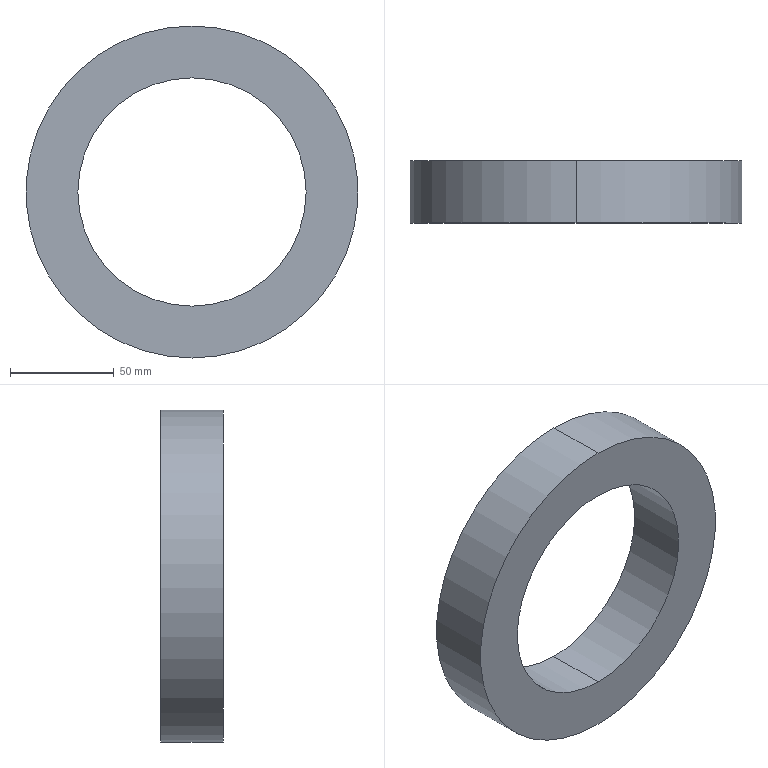Part | SolidWorks | features Extrusion 1, HoleWzd 1 | 1 solid | 30 faces | box 160 x 30 x 160 mm | volume 312871 mm3 | cone 16 | cylinder 12 | plane 2 | commonest cylinder face diameters 8.5 x8 110 x2 160 x2
STEP:
#1=CARTESIAN_POINT('',(65.,29.35,-4.25));
#2=VERTEX_POINT('',#1);
#3=CARTESIAN_POINT('',(65.,29.35,4.25));
#4=VERTEX_POINT('',#3);
#5=CARTESIAN_POINT('',(65.,29.35,0.));
#6=DIRECTION('',(0.,1.,0.));
#7=DIRECTION('',(0.,0.,1.));
#8=AXIS2_PLACEMENT_3D('',#5,#6,#7);
#9=CIRCLE('',#8,4.25);
#10=EDGE_CURVE('',#2,#4,#9,.T.);
#11=ORIENTED_EDGE('',*,*,#10,.F.);
#12=CARTESIAN_POINT('',(65.,30.,-5.025));
#13=VERTEX_POINT('',#12);
#14=CARTESIAN_POINT('',(65.,30.,-5.025));
#15=DIRECTION('',(0.,0.6428,-0.766));
#16=VECTOR('',#15,1000.);
#17=LINE('',#14,#16);
#18=EDGE_CURVE('',#2,#13,#17,.T.);
#19=ORIENTED_EDGE('',*,*,#18,.T.);
#20=CARTESIAN_POINT('',(65.,30.,5.025));
#21=VERTEX_POINT('',#20);
#22=CARTESIAN_POINT('',(65.,30.,0.));
#23=DIRECTION('',(0.,1.,0.));
#24=DIRECTION('',(0.,0.,1.));
#25=AXIS2_PLACEMENT_3D('',#22,#23,#24);
#26=CIRCLE('',#25,5.025);
#27=EDGE_CURVE('',#13,#21,#26,.T.);
#28=ORIENTED_EDGE('',*,*,#27,.T.);
#29=CARTESIAN_POINT('',(65.,30.,5.025));
#30=DIRECTION('',(0.,0.6428,0.766));
#31=VECTOR('',#30,1000.);
#32=LINE('',#29,#31);
#33=EDGE_CURVE('',#4,#21,#32,.T.);
#34=ORIENTED_EDGE('',*,*,#33,.F.);
#35=EDGE_LOOP('',(#11,#19,#28,#34));
#36=FACE_OUTER_BOUND('',#35,.T.);
#37=CARTESIAN_POINT('',(65.,30.,0.));
#38=DIRECTION('',(0.,1.,0.));
#39=DIRECTION('',(0.,0.,1.));
#40=AXIS2_PLACEMENT_3D('',#37,#38,#39);
#41=CONICAL_SURFACE('',#40,5.025,0.8727);
#42=ADVANCED_FACE('',(#36),#41,.F.);
#43=CARTESIAN_POINT('',(65.,8.,-4.25));
#44=VERTEX_POINT('',#43);
#45=CARTESIAN_POINT('',(65.,8.,4.25));
#46=VERTEX_POINT('',#45);
#47=CARTESIAN_POINT('',(65.,8.,0.));
#48=DIRECTION('',(0.,1.,0.));
#49=DIRECTION('',(0.,0.,1.));
#50=AXIS2_PLACEMENT_3D('',#47,#48,#49);
#51=CIRCLE('',#50,4.25);
#52=EDGE_CURVE('',#44,#46,#51,.T.);
#53=ORIENTED_EDGE('',*,*,#52,.F.);
#54=CARTESIAN_POINT('',(65.,30.,-4.25));
#55=DIRECTION('',(0.,1.,0.));
#56=VECTOR('',#55,1000.);
#57=LINE('',#54,#56);
#58=EDGE_CURVE('',#44,#2,#57,.T.);
#59=ORIENTED_EDGE('',*,*,#58,.T.);
#60=ORIENTED_EDGE('',*,*,#10,.T.);
#61=CARTESIAN_POINT('',(65.,30.,4.25));
#62=DIRECTION('',(0.,1.,0.));
#63=VECTOR('',#62,1000.);
#64=LINE('',#61,#63);
#65=EDGE_CURVE('',#46,#4,#64,.T.);
#66=ORIENTED_EDGE('',*,*,#65,.F.);
#67=EDGE_LOOP('',(#53,#59,#60,#66));
#68=FACE_OUTER_BOUND('',#67,.T.);
#69=CARTESIAN_POINT('',(65.,30.,0.));
#70=DIRECTION('',(0.,1.,0.));
#71=DIRECTION('',(0.,0.,1.));
#72=AXIS2_PLACEMENT_3D('',#69,#70,#71);
#73=CYLINDRICAL_SURFACE('',#72,4.25);
#74=ADVANCED_FACE('',(#68),#73,.F.);
#75=CARTESIAN_POINT('',(65.,5.446,0.));
#76=VERTEX_POINT('',#75);
#77=CARTESIAN_POINT('',(65.,8.,4.25));
#78=DIRECTION('',(0.,0.515,0.8572));
#79=VECTOR('',#78,1000.);
#80=LINE('',#77,#79);
#81=EDGE_CURVE('',#76,#46,#80,.T.);
#82=ORIENTED_EDGE('',*,*,#81,.F.);
#83=CARTESIAN_POINT('',(65.,8.,-4.25));
#84=DIRECTION('',(0.,0.515,-0.8572));
#85=VECTOR('',#84,1000.);
#86=LINE('',#83,#85);
#87=EDGE_CURVE('',#76,#44,#86,.T.);
#88=ORIENTED_EDGE('',*,*,#87,.T.);
#89=ORIENTED_EDGE('',*,*,#52,.T.);
#90=EDGE_LOOP('',(#82,#88,#89));
#91=FACE_OUTER_BOUND('',#90,.T.);
#92=CARTESIAN_POINT('',(65.,8.,0.));
#93=DIRECTION('',(0.,1.,0.));
#94=DIRECTION('',(0.,0.,1.));
#95=AXIS2_PLACEMENT_3D('',#92,#93,#94);
#96=CONICAL_SURFACE('',#95,4.25,1.03);
#97=ADVANCED_FACE('',(#91),#96,.F.);
#98=CARTESIAN_POINT('',(0.,29.35,60.75));
#99=VERTEX_POINT('',#98);
#100=CARTESIAN_POINT('',(0.,29.35,69.25));
#101=VERTEX_POINT('',#100);
#102=CARTESIAN_POINT('',(0.,29.35,65.));
#103=DIRECTION('',(0.,1.,0.));
#104=DIRECTION('',(0.,0.,1.));
#105=AXIS2_PLACEMENT_3D('',#102,#103,#104);
#106=CIRCLE('',#105,4.25);
#107=EDGE_CURVE('',#99,#101,#106,.T.);
#108=ORIENTED_EDGE('',*,*,#107,.F.);
#109=CARTESIAN_POINT('',(0.,30.,59.975));
#110=VERTEX_POINT('',#109);
#111=CARTESIAN_POINT('',(0.,30.,59.975));
#112=DIRECTION('',(0.,0.6428,-0.766));
#113=VECTOR('',#112,1000.);
#114=LINE('',#111,#113);
#115=EDGE_CURVE('',#99,#110,#114,.T.);
#116=ORIENTED_EDGE('',*,*,#115,.T.);
#117=CARTESIAN_POINT('',(0.,30.,70.025));
#118=VERTEX_POINT('',#117);
#119=CARTESIAN_POINT('',(0.,30.,65.));
#120=DIRECTION('',(0.,1.,0.));
#121=DIRECTION('',(0.,0.,1.));
#122=AXIS2_PLACEMENT_3D('',#119,#120,#121);
#123=CIRCLE('',#122,5.025);
#124=EDGE_CURVE('',#110,#118,#123,.T.);
#125=ORIENTED_EDGE('',*,*,#124,.T.);
#126=CARTESIAN_POINT('',(0.,30.,70.025));
#127=DIRECTION('',(0.,0.6428,0.766));
#128=VECTOR('',#127,1000.);
#129=LINE('',#126,#128);
#130=EDGE_CURVE('',#101,#118,#129,.T.);
#131=ORIENTED_EDGE('',*,*,#130,.F.);
#132=EDGE_LOOP('',(#108,#116,#125,#131));
#133=FACE_OUTER_BOUND('',#132,.T.);
#134=CARTESIAN_POINT('',(0.,30.,65.));
#135=DIRECTION('',(0.,1.,0.));
#136=DIRECTION('',(0.,0.,1.));
#137=AXIS2_PLACEMENT_3D('',#134,#135,#136);
#138=CONICAL_SURFACE('',#137,5.025,0.8727);
#139=ADVANCED_FACE('',(#133),#138,.F.);
#140=CARTESIAN_POINT('',(0.,8.,60.75));
#141=VERTEX_POINT('',#140);
#142=CARTESIAN_POINT('',(0.,8.,69.25));
#143=VERTEX_POINT('',#142);
#144=CARTESIAN_POINT('',(0.,8.,65.));
#145=DIRECTION('',(0.,1.,0.));
#146=DIRECTION('',(0.,0.,1.));
#147=AXIS2_PLACEMENT_3D('',#144,#145,#146);
#148=CIRCLE('',#147,4.25);
#149=EDGE_CURVE('',#141,#143,#148,.T.);
#150=ORIENTED_EDGE('',*,*,#149,.F.);
#151=CARTESIAN_POINT('',(0.,30.,60.75));
#152=DIRECTION('',(0.,1.,0.));
#153=VECTOR('',#152,1000.);
#154=LINE('',#151,#153);
#155=EDGE_CURVE('',#141,#99,#154,.T.);
#156=ORIENTED_EDGE('',*,*,#155,.T.);
#157=ORIENTED_EDGE('',*,*,#107,.T.);
#158=CARTESIAN_POINT('',(0.,30.,69.25));
#159=DIRECTION('',(0.,1.,0.));
#160=VECTOR('',#159,1000.);
#161=LINE('',#158,#160);
#162=EDGE_CURVE('',#143,#101,#161,.T.);
#163=ORIENTED_EDGE('',*,*,#162,.F.);
#164=EDGE_LOOP('',(#150,#156,#157,#163));
#165=FACE_OUTER_BOUND('',#164,.T.);
#166=CARTESIAN_POINT('',(0.,30.,65.));
#167=DIRECTION('',(0.,1.,0.));
#168=DIRECTION('',(0.,0.,1.));
#169=AXIS2_PLACEMENT_3D('',#166,#167,#168);
#170=CYLINDRICAL_SURFACE('',#169,4.25);
#171=ADVANCED_FACE('',(#165),#170,.F.);
#172=CARTESIAN_POINT('',(0.,5.446,65.));
#173=VERTEX_POINT('',#172);
#174=CARTESIAN_POINT('',(0.,8.,69.25));
#175=DIRECTION('',(0.,0.515,0.8572));
#176=VECTOR('',#175,1000.);
#177=LINE('',#174,#176);
#178=EDGE_CURVE('',#173,#143,#177,.T.);
#179=ORIENTED_EDGE('',*,*,#178,.F.);
#180=CARTESIAN_POINT('',(0.,8.,60.75));
#181=DIRECTION('',(0.,0.515,-0.8572));
#182=VECTOR('',#181,1000.);
#183=LINE('',#180,#182);
#184=EDGE_CURVE('',#173,#141,#183,.T.);
#185=ORIENTED_EDGE('',*,*,#184,.T.);
#186=ORIENTED_EDGE('',*,*,#149,.T.);
#187=EDGE_LOOP('',(#179,#185,#186));
#188=FACE_OUTER_BOUND('',#187,.T.);
#189=CARTESIAN_POINT('',(0.,8.,65.));
#190=DIRECTION('',(0.,1.,0.));
#191=DIRECTION('',(0.,0.,1.));
#192=AXIS2_PLACEMENT_3D('',#189,#190,#191);
#193=CONICAL_SURFACE('',#192,4.25,1.03);
#194=ADVANCED_FACE('',(#188),#193,.F.);
#195=CARTESIAN_POINT('',(-65.,29.35,-4.25));
#196=VERTEX_POINT('',#195);
#197=CARTESIAN_POINT('',(-65.,29.35,4.25));
#198=VERTEX_POINT('',#197);
#199=CARTESIAN_POINT('',(-65.,29.35,0.));
#200=DIRECTION('',(0.,1.,0.));
#201=DIRECTION('',(0.,0.,1.));
#202=AXIS2_PLACEMENT_3D('',#199,#200,#201);
#203=CIRCLE('',#202,4.25);
#204=EDGE_CURVE('',#196,#198,#203,.T.);
#205=ORIENTED_EDGE('',*,*,#204,.F.);
#206=CARTESIAN_POINT('',(-65.,30.,-5.025));
#207=VERTEX_POINT('',#206);
#208=CARTESIAN_POINT('',(-65.,30.,-5.025));
#209=DIRECTION('',(0.,0.6428,-0.766));
#210=VECTOR('',#209,1000.);
#211=LINE('',#208,#210);
#212=EDGE_CURVE('',#196,#207,#211,.T.);
#213=ORIENTED_EDGE('',*,*,#212,.T.);
#214=CARTESIAN_POINT('',(-65.,30.,5.025));
#215=VERTEX_POINT('',#214);
#216=CARTESIAN_POINT('',(-65.,30.,0.));
#217=DIRECTION('',(0.,1.,0.));
#218=DIRECTION('',(0.,0.,1.));
#219=AXIS2_PLACEMENT_3D('',#216,#217,#218);
#220=CIRCLE('',#219,5.025);
#221=EDGE_CURVE('',#207,#215,#220,.T.);
#222=ORIENTED_EDGE('',*,*,#221,.T.);
#223=CARTESIAN_POINT('',(-65.,30.,5.025));
#224=DIRECTION('',(0.,0.6428,0.766));
#225=VECTOR('',#224,1000.);
#226=LINE('',#223,#225);
#227=EDGE_CURVE('',#198,#215,#226,.T.);
#228=ORIENTED_EDGE('',*,*,#227,.F.);
#229=EDGE_LOOP('',(#205,#213,#222,#228));
#230=FACE_OUTER_BOUND('',#229,.T.);
#231=CARTESIAN_POINT('',(-65.,30.,0.));
#232=DIRECTION('',(0.,1.,0.));
#233=DIRECTION('',(0.,0.,1.));
#234=AXIS2_PLACEMENT_3D('',#231,#232,#233);
#235=CONICAL_SURFACE('',#234,5.025,0.8727);
#236=ADVANCED_FACE('',(#230),#235,.F.);
#237=CARTESIAN_POINT('',(-65.,8.,-4.25));
#238=VERTEX_POINT('',#237);
#239=CARTESIAN_POINT('',(-65.,8.,4.25));
#240=VERTEX_POINT('',#239);
#241=CARTESIAN_POINT('',(-65.,8.,0.));
#242=DIRECTION('',(0.,1.,0.));
#243=DIRECTION('',(0.,0.,1.));
#244=AXIS2_PLACEMENT_3D('',#241,#242,#243);
#245=CIRCLE('',#244,4.25);
#246=EDGE_CURVE('',#238,#240,#245,.T.);
#247=ORIENTED_EDGE('',*,*,#246,.F.);
#248=CARTESIAN_POINT('',(-65.,30.,-4.25));
#249=DIRECTION('',(0.,1.,0.));
#250=VECTOR('',#249,1000.);
#251=LINE('',#248,#250);
#252=EDGE_CURVE('',#238,#196,#251,.T.);
#253=ORIENTED_EDGE('',*,*,#252,.T.);
#254=ORIENTED_EDGE('',*,*,#204,.T.);
#255=CARTESIAN_POINT('',(-65.,30.,4.25));
#256=DIRECTION('',(0.,1.,0.));
#257=VECTOR('',#256,1000.);
#258=LINE('',#255,#257);
#259=EDGE_CURVE('',#240,#198,#258,.T.);
#260=ORIENTED_EDGE('',*,*,#259,.F.);
#261=EDGE_LOOP('',(#247,#253,#254,#260));
#262=FACE_OUTER_BOUND('',#261,.T.);
#263=CARTESIAN_POINT('',(-65.,30.,0.));
#264=DIRECTION('',(0.,1.,0.));
#265=DIRECTION('',(0.,0.,1.));
#266=AXIS2_PLACEMENT_3D('',#263,#264,#265);
#267=CYLINDRICAL_SURFACE('',#266,4.25);
#268=ADVANCED_FACE('',(#262),#267,.F.);
#269=CARTESIAN_POINT('',(-65.,5.446,0.));
#270=VERTEX_POINT('',#269);
#271=CARTESIAN_POINT('',(-65.,8.,4.25));
#272=DIRECTION('',(0.,0.515,0.8572));
#273=VECTOR('',#272,1000.);
#274=LINE('',#271,#273);
#275=EDGE_CURVE('',#270,#240,#274,.T.);
#276=ORIENTED_EDGE('',*,*,#275,.F.);
#277=CARTESIAN_POINT('',(-65.,8.,-4.25));
#278=DIRECTION('',(0.,0.515,-0.8572));
#279=VECTOR('',#278,1000.);
#280=LINE('',#277,#279);
#281=EDGE_CURVE('',#270,#238,#280,.T.);
#282=ORIENTED_EDGE('',*,*,#281,.T.);
#283=ORIENTED_EDGE('',*,*,#246,.T.);
#284=EDGE_LOOP('',(#276,#282,#283));
#285=FACE_OUTER_BOUND('',#284,.T.);
#286=CARTESIAN_POINT('',(-65.,8.,0.));
#287=DIRECTION('',(0.,1.,0.));
#288=DIRECTION('',(0.,0.,1.));
#289=AXIS2_PLACEMENT_3D('',#286,#287,#288);
#290=CONICAL_SURFACE('',#289,4.25,1.03);
#291=ADVANCED_FACE('',(#285),#290,.F.);
#292=CARTESIAN_POINT('',(0.,29.35,-69.25));
#293=VERTEX_POINT('',#292);
#294=CARTESIAN_POINT('',(0.,29.35,-60.75));
#295=VERTEX_POINT('',#294);
#296=CARTESIAN_POINT('',(0.,29.35,-65.));
#297=DIRECTION('',(0.,1.,0.));
#298=DIRECTION('',(0.,0.,1.));
#299=AXIS2_PLACEMENT_3D('',#296,#297,#298);
#300=CIRCLE('',#299,4.25);
#301=EDGE_CURVE('',#293,#295,#300,.T.);
#302=ORIENTED_EDGE('',*,*,#301,.F.);
#303=CARTESIAN_POINT('',(0.,30.,-70.025));
#304=VERTEX_POINT('',#303);
#305=CARTESIAN_POINT('',(0.,30.,-70.025));
#306=DIRECTION('',(0.,0.6428,-0.766));
#307=VECTOR('',#306,1000.);
#308=LINE('',#305,#307);
#309=EDGE_CURVE('',#293,#304,#308,.T.);
#310=ORIENTED_EDGE('',*,*,#309,.T.);
#311=CARTESIAN_POINT('',(0.,30.,-59.975));
#312=VERTEX_POINT('',#311);
#313=CARTESIAN_POINT('',(0.,30.,-65.));
#314=DIRECTION('',(0.,1.,0.));
#315=DIRECTION('',(0.,0.,1.));
#316=AXIS2_PLACEMENT_3D('',#313,#314,#315);
#317=CIRCLE('',#316,5.025);
#318=EDGE_CURVE('',#304,#312,#317,.T.);
#319=ORIENTED_EDGE('',*,*,#318,.T.);
#320=CARTESIAN_POINT('',(0.,30.,-59.975));
#321=DIRECTION('',(0.,0.6428,0.766));
#322=VECTOR('',#321,1000.);
#323=LINE('',#320,#322);
#324=EDGE_CURVE('',#295,#312,#323,.T.);
#325=ORIENTED_EDGE('',*,*,#324,.F.);
#326=EDGE_LOOP('',(#302,#310,#319,#325));
#327=FACE_OUTER_BOUND('',#326,.T.);
#328=CARTESIAN_POINT('',(0.,30.,-65.));
#329=DIRECTION('',(0.,1.,0.));
#330=DIRECTION('',(0.,0.,1.));
#331=AXIS2_PLACEMENT_3D('',#328,#329,#330);
#332=CONICAL_SURFACE('',#331,5.025,0.8727);
#333=ADVANCED_FACE('',(#327),#332,.F.);
#334=CARTESIAN_POINT('',(0.,8.,-69.25));
#335=VERTEX_POINT('',#334);
#336=CARTESIAN_POINT('',(0.,8.,-60.75));
#337=VERTEX_POINT('',#336);
#338=CARTESIAN_POINT('',(0.,8.,-65.));
#339=DIRECTION('',(0.,1.,0.));
#340=DIRECTION('',(0.,0.,1.));
#341=AXIS2_PLACEMENT_3D('',#338,#339,#340);
#342=CIRCLE('',#341,4.25);
#343=EDGE_CURVE('',#335,#337,#342,.T.);
#344=ORIENTED_EDGE('',*,*,#343,.F.);
#345=CARTESIAN_POINT('',(0.,30.,-69.25));
#346=DIRECTION('',(0.,1.,0.));
#347=VECTOR('',#346,1000.);
#348=LINE('',#345,#347);
#349=EDGE_CURVE('',#335,#293,#348,.T.);
#350=ORIENTED_EDGE('',*,*,#349,.T.);
#351=ORIENTED_EDGE('',*,*,#301,.T.);
#352=CARTESIAN_POINT('',(0.,30.,-60.75));
#353=DIRECTION('',(0.,1.,0.));
#354=VECTOR('',#353,1000.);
#355=LINE('',#352,#354);
#356=EDGE_CURVE('',#337,#295,#355,.T.);
#357=ORIENTED_EDGE('',*,*,#356,.F.);
#358=EDGE_LOOP('',(#344,#350,#351,#357));
#359=FACE_OUTER_BOUND('',#358,.T.);
#360=CARTESIAN_POINT('',(0.,30.,-65.));
#361=DIRECTION('',(0.,1.,0.));
#362=DIRECTION('',(0.,0.,1.));
#363=AXIS2_PLACEMENT_3D('',#360,#361,#362);
#364=CYLINDRICAL_SURFACE('',#363,4.25);
#365=ADVANCED_FACE('',(#359),#364,.F.);
#366=CARTESIAN_POINT('',(0.,5.446,-65.));
#367=VERTEX_POINT('',#366);
#368=CARTESIAN_POINT('',(0.,8.,-60.75));
#369=DIRECTION('',(0.,0.515,0.8572));
#370=VECTOR('',#369,1000.);
#371=LINE('',#368,#370);
#372=EDGE_CURVE('',#367,#337,#371,.T.);
#373=ORIENTED_EDGE('',*,*,#372,.F.);
#374=CARTESIAN_POINT('',(0.,8.,-69.25));
#375=DIRECTION('',(0.,0.515,-0.8572));
#376=VECTOR('',#375,1000.);
#377=LINE('',#374,#376);
#378=EDGE_CURVE('',#367,#335,#377,.T.);
#379=ORIENTED_EDGE('',*,*,#378,.T.);
#380=ORIENTED_EDGE('',*,*,#343,.T.);
#381=EDGE_LOOP('',(#373,#379,#380));
#382=FACE_OUTER_BOUND('',#381,.T.);
#383=CARTESIAN_POINT('',(0.,8.,-65.));
#384=DIRECTION('',(0.,1.,0.));
#385=DIRECTION('',(0.,0.,1.));
#386=AXIS2_PLACEMENT_3D('',#383,#384,#385);
#387=CONICAL_SURFACE('',#386,4.25,1.03);
#388=ADVANCED_FACE('',(#382),#387,.F.);
#389=CARTESIAN_POINT('',(0.,30.,-55.));
#390=VERTEX_POINT('',#389);
#391=CARTESIAN_POINT('',(0.,30.,55.));
#392=VERTEX_POINT('',#391);
#393=CARTESIAN_POINT('',(0.,30.,0.));
#394=DIRECTION('',(0.,1.,0.));
#395=DIRECTION('',(0.,0.,1.));
#396=AXIS2_PLACEMENT_3D('',#393,#394,#395);
#397=CIRCLE('',#396,55.);
#398=EDGE_CURVE('',#390,#392,#397,.T.);
#399=ORIENTED_EDGE('',*,*,#398,.T.);
#400=CARTESIAN_POINT('',(0.,0.,55.));
#401=VERTEX_POINT('',#400);
#402=CARTESIAN_POINT('',(0.,30.,55.));
#403=DIRECTION('',(0.,-1.,0.));
#404=VECTOR('',#403,1000.);
#405=LINE('',#402,#404);
#406=EDGE_CURVE('',#392,#401,#405,.T.);
#407=ORIENTED_EDGE('',*,*,#406,.T.);
#408=CARTESIAN_POINT('',(0.,0.,-55.));
#409=VERTEX_POINT('',#408);
#410=CARTESIAN_POINT('',(0.,0.,0.));
#411=DIRECTION('',(0.,1.,0.));
#412=DIRECTION('',(0.,0.,1.));
#413=AXIS2_PLACEMENT_3D('',#410,#411,#412);
#414=CIRCLE('',#413,55.);
#415=EDGE_CURVE('',#409,#401,#414,.T.);
#416=ORIENTED_EDGE('',*,*,#415,.F.);
#417=CARTESIAN_POINT('',(0.,30.,-55.));
#418=DIRECTION('',(0.,-1.,0.));
#419=VECTOR('',#418,1000.);
#420=LINE('',#417,#419);
#421=EDGE_CURVE('',#390,#409,#420,.T.);
#422=ORIENTED_EDGE('',*,*,#421,.F.);
#423=EDGE_LOOP('',(#399,#407,#416,#422));
#424=FACE_OUTER_BOUND('',#423,.T.);
#425=CARTESIAN_POINT('',(0.,30.,0.));
#426=DIRECTION('',(0.,-1.,0.));
#427=DIRECTION('',(0.,0.,-1.));
#428=AXIS2_PLACEMENT_3D('',#425,#426,#427);
#429=CYLINDRICAL_SURFACE('',#428,55.);
#430=ADVANCED_FACE('',(#424),#429,.F.);
#431=CARTESIAN_POINT('',(0.,30.,80.));
#432=VERTEX_POINT('',#431);
#433=CARTESIAN_POINT('',(0.,30.,-80.));
#434=VERTEX_POINT('',#433);
#435=CARTESIAN_POINT('',(0.,30.,0.));
#436=DIRECTION('',(0.,1.,0.));
#437=DIRECTION('',(0.,0.,1.));
#438=AXIS2_PLACEMENT_3D('',#435,#436,#437);
#439=CIRCLE('',#438,80.);
#440=EDGE_CURVE('',#432,#434,#439,.T.);
#441=ORIENTED_EDGE('',*,*,#440,.F.);
#442=CARTESIAN_POINT('',(0.,0.,80.));
#443=VERTEX_POINT('',#442);
#444=CARTESIAN_POINT('',(0.,30.,80.));
#445=DIRECTION('',(0.,-1.,0.));
#446=VECTOR('',#445,1000.);
#447=LINE('',#444,#446);
#448=EDGE_CURVE('',#432,#443,#447,.T.);
#449=ORIENTED_EDGE('',*,*,#448,.T.);
#450=CARTESIAN_POINT('',(0.,0.,-80.));
#451=VERTEX_POINT('',#450);
#452=CARTESIAN_POINT('',(0.,0.,0.));
#453=DIRECTION('',(0.,1.,0.));
#454=DIRECTION('',(0.,0.,1.));
#455=AXIS2_PLACEMENT_3D('',#452,#453,#454);
#456=CIRCLE('',#455,80.);
#457=EDGE_CURVE('',#443,#451,#456,.T.);
#458=ORIENTED_EDGE('',*,*,#457,.T.);
#459=CARTESIAN_POINT('',(0.,30.,-80.));
#460=DIRECTION('',(0.,-1.,0.));
#461=VECTOR('',#460,1000.);
#462=LINE('',#459,#461);
#463=EDGE_CURVE('',#434,#451,#462,.T.);
#464=ORIENTED_EDGE('',*,*,#463,.F.);
#465=EDGE_LOOP('',(#441,#449,#458,#464));
#466=FACE_OUTER_BOUND('',#465,.T.);
#467=CARTESIAN_POINT('',(0.,30.,0.));
#468=DIRECTION('',(0.,-1.,0.));
#469=DIRECTION('',(0.,0.,-1.));
#470=AXIS2_PLACEMENT_3D('',#467,#468,#469);
#471=CYLINDRICAL_SURFACE('',#470,80.);
#472=ADVANCED_FACE('',(#466),#471,.T.);
#473=CARTESIAN_POINT('',(65.,30.,0.));
#474=DIRECTION('',(0.,1.,0.));
#475=DIRECTION('',(0.,0.,1.));
#476=AXIS2_PLACEMENT_3D('',#473,#474,#475);
#477=CIRCLE('',#476,5.025);
#478=EDGE_CURVE('',#21,#13,#477,.T.);
#479=ORIENTED_EDGE('',*,*,#478,.F.);
#480=ORIENTED_EDGE('',*,*,#27,.F.);
#481=EDGE_LOOP('',(#479,#480));
#482=FACE_BOUND('',#481,.T.);
#483=CARTESIAN_POINT('',(0.,30.,65.));
#484=DIRECTION('',(0.,1.,0.));
#485=DIRECTION('',(0.,0.,1.));
#486=AXIS2_PLACEMENT_3D('',#483,#484,#485);
#487=CIRCLE('',#486,5.025);
#488=EDGE_CURVE('',#118,#110,#487,.T.);
#489=ORIENTED_EDGE('',*,*,#488,.F.);
#490=ORIENTED_EDGE('',*,*,#124,.F.);
#491=EDGE_LOOP('',(#489,#490));
#492=FACE_BOUND('',#491,.T.);
#493=CARTESIAN_POINT('',(-65.,30.,0.));
#494=DIRECTION('',(0.,1.,0.));
#495=DIRECTION('',(0.,0.,1.));
#496=AXIS2_PLACEMENT_3D('',#493,#494,#495);
#497=CIRCLE('',#496,5.025);
#498=EDGE_CURVE('',#215,#207,#497,.T.);
#499=ORIENTED_EDGE('',*,*,#498,.F.);
#500=ORIENTED_EDGE('',*,*,#221,.F.);
#501=EDGE_LOOP('',(#499,#500));
#502=FACE_BOUND('',#501,.T.);
#503=CARTESIAN_POINT('',(0.,30.,-65.));
#504=DIRECTION('',(0.,1.,0.));
#505=DIRECTION('',(0.,0.,1.));
#506=AXIS2_PLACEMENT_3D('',#503,#504,#505);
#507=CIRCLE('',#506,5.025);
#508=EDGE_CURVE('',#312,#304,#507,.T.);
#509=ORIENTED_EDGE('',*,*,#508,.F.);
#510=ORIENTED_EDGE('',*,*,#318,.F.);
#511=EDGE_LOOP('',(#509,#510));
#512=FACE_BOUND('',#511,.T.);
#513=CARTESIAN_POINT('',(0.,30.,0.));
#514=DIRECTION('',(0.,1.,0.));
#515=DIRECTION('',(0.,0.,1.));
#516=AXIS2_PLACEMENT_3D('',#513,#514,#515);
#517=CIRCLE('',#516,80.);
#518=EDGE_CURVE('',#434,#432,#517,.T.);
#519=ORIENTED_EDGE('',*,*,#518,.T.);
#520=ORIENTED_EDGE('',*,*,#440,.T.);
#521=EDGE_LOOP('',(#519,#520));
#522=FACE_OUTER_BOUND('',#521,.T.);
#523=ORIENTED_EDGE('',*,*,#398,.F.);
#524=CARTESIAN_POINT('',(0.,30.,0.));
#525=DIRECTION('',(0.,1.,0.));
#526=DIRECTION('',(0.,0.,1.));
#527=AXIS2_PLACEMENT_3D('',#524,#525,#526);
#528=CIRCLE('',#527,55.);
#529=EDGE_CURVE('',#392,#390,#528,.T.);
#530=ORIENTED_EDGE('',*,*,#529,.F.);
#531=EDGE_LOOP('',(#523,#530));
#532=FACE_BOUND('',#531,.T.);
#533=CARTESIAN_POINT('',(0.,30.,0.));
#534=DIRECTION('',(0.,1.,0.));
#535=DIRECTION('',(0.,0.,1.));
#536=AXIS2_PLACEMENT_3D('',#533,#534,#535);
#537=PLANE('',#536);
#538=ADVANCED_FACE('',(#482,#492,#502,#512,#522,#532),#537,.T.);
#539=CARTESIAN_POINT('',(0.,0.,0.));
#540=DIRECTION('',(0.,1.,0.));
#541=DIRECTION('',(0.,0.,1.));
#542=AXIS2_PLACEMENT_3D('',#539,#540,#541);
#543=CIRCLE('',#542,80.);
#544=EDGE_CURVE('',#451,#443,#543,.T.);
#545=ORIENTED_EDGE('',*,*,#544,.F.);
#546=ORIENTED_EDGE('',*,*,#457,.F.);
#547=EDGE_LOOP('',(#545,#546));
#548=FACE_OUTER_BOUND('',#547,.T.);
#549=ORIENTED_EDGE('',*,*,#415,.T.);
#550=CARTESIAN_POINT('',(0.,0.,0.));
#551=DIRECTION('',(0.,1.,0.));
#552=DIRECTION('',(0.,0.,1.));
#553=AXIS2_PLACEMENT_3D('',#550,#551,#552);
#554=CIRCLE('',#553,55.);
#555=EDGE_CURVE('',#401,#409,#554,.T.);
#556=ORIENTED_EDGE('',*,*,#555,.T.);
#557=EDGE_LOOP('',(#549,#556));
#558=FACE_BOUND('',#557,.T.);
#559=CARTESIAN_POINT('',(0.,0.,0.));
#560=DIRECTION('',(0.,1.,0.));
#561=DIRECTION('',(0.,0.,1.));
#562=AXIS2_PLACEMENT_3D('',#559,#560,#561);
#563=PLANE('',#562);
#564=ADVANCED_FACE('',(#548,#558),#563,.F.);
#565=ORIENTED_EDGE('',*,*,#448,.F.);
#566=ORIENTED_EDGE('',*,*,#518,.F.);
#567=ORIENTED_EDGE('',*,*,#463,.T.);
#568=ORIENTED_EDGE('',*,*,#544,.T.);
#569=EDGE_LOOP('',(#565,#566,#567,#568));
#570=FACE_OUTER_BOUND('',#569,.T.);
#571=CARTESIAN_POINT('',(0.,30.,0.));
#572=DIRECTION('',(0.,-1.,0.));
#573=DIRECTION('',(0.,0.,-1.));
#574=AXIS2_PLACEMENT_3D('',#571,#572,#573);
#575=CYLINDRICAL_SURFACE('',#574,80.);
#576=ADVANCED_FACE('',(#570),#575,.T.);
#577=ORIENTED_EDGE('',*,*,#406,.F.);
#578=ORIENTED_EDGE('',*,*,#529,.T.);
#579=ORIENTED_EDGE('',*,*,#421,.T.);
#580=ORIENTED_EDGE('',*,*,#555,.F.);
#581=EDGE_LOOP('',(#577,#578,#579,#580));
#582=FACE_OUTER_BOUND('',#581,.T.);
#583=CARTESIAN_POINT('',(0.,30.,0.));
#584=DIRECTION('',(0.,-1.,0.));
#585=DIRECTION('',(0.,0.,-1.));
#586=AXIS2_PLACEMENT_3D('',#583,#584,#585);
#587=CYLINDRICAL_SURFACE('',#586,55.);
#588=ADVANCED_FACE('',(#582),#587,.F.);
#589=ORIENTED_EDGE('',*,*,#378,.F.);
#590=ORIENTED_EDGE('',*,*,#372,.T.);
#591=CARTESIAN_POINT('',(0.,8.,-65.));
#592=DIRECTION('',(0.,1.,0.));
#593=DIRECTION('',(0.,0.,1.));
#594=AXIS2_PLACEMENT_3D('',#591,#592,#593);
#595=CIRCLE('',#594,4.25);
#596=EDGE_CURVE('',#337,#335,#595,.T.);
#597=ORIENTED_EDGE('',*,*,#596,.T.);
#598=EDGE_LOOP('',(#589,#590,#597));
#599=FACE_OUTER_BOUND('',#598,.T.);
#600=CARTESIAN_POINT('',(0.,8.,-65.));
#601=DIRECTION('',(0.,1.,0.));
#602=DIRECTION('',(0.,0.,1.));
#603=AXIS2_PLACEMENT_3D('',#600,#601,#602);
#604=CONICAL_SURFACE('',#603,4.25,1.03);
#605=ADVANCED_FACE('',(#599),#604,.F.);
#606=ORIENTED_EDGE('',*,*,#349,.F.);
#607=ORIENTED_EDGE('',*,*,#596,.F.);
#608=ORIENTED_EDGE('',*,*,#356,.T.);
#609=CARTESIAN_POINT('',(0.,29.35,-65.));
#610=DIRECTION('',(0.,1.,0.));
#611=DIRECTION('',(0.,0.,1.));
#612=AXIS2_PLACEMENT_3D('',#609,#610,#611);
#613=CIRCLE('',#612,4.25);
#614=EDGE_CURVE('',#295,#293,#613,.T.);
#615=ORIENTED_EDGE('',*,*,#614,.T.);
#616=EDGE_LOOP('',(#606,#607,#608,#615));
#617=FACE_OUTER_BOUND('',#616,.T.);
#618=CARTESIAN_POINT('',(0.,30.,-65.));
#619=DIRECTION('',(0.,1.,0.));
#620=DIRECTION('',(0.,0.,1.));
#621=AXIS2_PLACEMENT_3D('',#618,#619,#620);
#622=CYLINDRICAL_SURFACE('',#621,4.25);
#623=ADVANCED_FACE('',(#617),#622,.F.);
#624=ORIENTED_EDGE('',*,*,#309,.F.);
#625=ORIENTED_EDGE('',*,*,#614,.F.);
#626=ORIENTED_EDGE('',*,*,#324,.T.);
#627=ORIENTED_EDGE('',*,*,#508,.T.);
#628=EDGE_LOOP('',(#624,#625,#626,#627));
#629=FACE_OUTER_BOUND('',#628,.T.);
#630=CARTESIAN_POINT('',(0.,30.,-65.));
#631=DIRECTION('',(0.,1.,0.));
#632=DIRECTION('',(0.,0.,1.));
#633=AXIS2_PLACEMENT_3D('',#630,#631,#632);
#634=CONICAL_SURFACE('',#633,5.025,0.8727);
#635=ADVANCED_FACE('',(#629),#634,.F.);
#636=ORIENTED_EDGE('',*,*,#281,.F.);
#637=ORIENTED_EDGE('',*,*,#275,.T.);
#638=CARTESIAN_POINT('',(-65.,8.,0.));
#639=DIRECTION('',(0.,1.,0.));
#640=DIRECTION('',(0.,0.,1.));
#641=AXIS2_PLACEMENT_3D('',#638,#639,#640);
#642=CIRCLE('',#641,4.25);
#643=EDGE_CURVE('',#240,#238,#642,.T.);
#644=ORIENTED_EDGE('',*,*,#643,.T.);
#645=EDGE_LOOP('',(#636,#637,#644));
#646=FACE_OUTER_BOUND('',#645,.T.);
#647=CARTESIAN_POINT('',(-65.,8.,0.));
#648=DIRECTION('',(0.,1.,0.));
#649=DIRECTION('',(0.,0.,1.));
#650=AXIS2_PLACEMENT_3D('',#647,#648,#649);
#651=CONICAL_SURFACE('',#650,4.25,1.03);
#652=ADVANCED_FACE('',(#646),#651,.F.);
#653=ORIENTED_EDGE('',*,*,#252,.F.);
#654=ORIENTED_EDGE('',*,*,#643,.F.);
#655=ORIENTED_EDGE('',*,*,#259,.T.);
#656=CARTESIAN_POINT('',(-65.,29.35,0.));
#657=DIRECTION('',(0.,1.,0.));
#658=DIRECTION('',(0.,0.,1.));
#659=AXIS2_PLACEMENT_3D('',#656,#657,#658);
#660=CIRCLE('',#659,4.25);
#661=EDGE_CURVE('',#198,#196,#660,.T.);
#662=ORIENTED_EDGE('',*,*,#661,.T.);
#663=EDGE_LOOP('',(#653,#654,#655,#662));
#664=FACE_OUTER_BOUND('',#663,.T.);
#665=CARTESIAN_POINT('',(-65.,30.,0.));
#666=DIRECTION('',(0.,1.,0.));
#667=DIRECTION('',(0.,0.,1.));
#668=AXIS2_PLACEMENT_3D('',#665,#666,#667);
#669=CYLINDRICAL_SURFACE('',#668,4.25);
#670=ADVANCED_FACE('',(#664),#669,.F.);
#671=ORIENTED_EDGE('',*,*,#212,.F.);
#672=ORIENTED_EDGE('',*,*,#661,.F.);
#673=ORIENTED_EDGE('',*,*,#227,.T.);
#674=ORIENTED_EDGE('',*,*,#498,.T.);
#675=EDGE_LOOP('',(#671,#672,#673,#674));
#676=FACE_OUTER_BOUND('',#675,.T.);
#677=CARTESIAN_POINT('',(-65.,30.,0.));
#678=DIRECTION('',(0.,1.,0.));
#679=DIRECTION('',(0.,0.,1.));
#680=AXIS2_PLACEMENT_3D('',#677,#678,#679);
#681=CONICAL_SURFACE('',#680,5.025,0.8727);
#682=ADVANCED_FACE('',(#676),#681,.F.);
#683=ORIENTED_EDGE('',*,*,#184,.F.);
#684=ORIENTED_EDGE('',*,*,#178,.T.);
#685=CARTESIAN_POINT('',(0.,8.,65.));
#686=DIRECTION('',(0.,1.,0.));
#687=DIRECTION('',(0.,0.,1.));
#688=AXIS2_PLACEMENT_3D('',#685,#686,#687);
#689=CIRCLE('',#688,4.25);
#690=EDGE_CURVE('',#143,#141,#689,.T.);
#691=ORIENTED_EDGE('',*,*,#690,.T.);
#692=EDGE_LOOP('',(#683,#684,#691));
#693=FACE_OUTER_BOUND('',#692,.T.);
#694=CARTESIAN_POINT('',(0.,8.,65.));
#695=DIRECTION('',(0.,1.,0.));
#696=DIRECTION('',(0.,0.,1.));
#697=AXIS2_PLACEMENT_3D('',#694,#695,#696);
#698=CONICAL_SURFACE('',#697,4.25,1.03);
#699=ADVANCED_FACE('',(#693),#698,.F.);
#700=ORIENTED_EDGE('',*,*,#155,.F.);
#701=ORIENTED_EDGE('',*,*,#690,.F.);
#702=ORIENTED_EDGE('',*,*,#162,.T.);
#703=CARTESIAN_POINT('',(0.,29.35,65.));
#704=DIRECTION('',(0.,1.,0.));
#705=DIRECTION('',(0.,0.,1.));
#706=AXIS2_PLACEMENT_3D('',#703,#704,#705);
#707=CIRCLE('',#706,4.25);
#708=EDGE_CURVE('',#101,#99,#707,.T.);
#709=ORIENTED_EDGE('',*,*,#708,.T.);
#710=EDGE_LOOP('',(#700,#701,#702,#709));
#711=FACE_OUTER_BOUND('',#710,.T.);
#712=CARTESIAN_POINT('',(0.,30.,65.));
#713=DIRECTION('',(0.,1.,0.));
#714=DIRECTION('',(0.,0.,1.));
#715=AXIS2_PLACEMENT_3D('',#712,#713,#714);
#716=CYLINDRICAL_SURFACE('',#715,4.25);
#717=ADVANCED_FACE('',(#711),#716,.F.);
#718=ORIENTED_EDGE('',*,*,#115,.F.);
#719=ORIENTED_EDGE('',*,*,#708,.F.);
#720=ORIENTED_EDGE('',*,*,#130,.T.);
#721=ORIENTED_EDGE('',*,*,#488,.T.);
#722=EDGE_LOOP('',(#718,#719,#720,#721));
#723=FACE_OUTER_BOUND('',#722,.T.);
#724=CARTESIAN_POINT('',(0.,30.,65.));
#725=DIRECTION('',(0.,1.,0.));
#726=DIRECTION('',(0.,0.,1.));
#727=AXIS2_PLACEMENT_3D('',#724,#725,#726);
#728=CONICAL_SURFACE('',#727,5.025,0.8727);
#729=ADVANCED_FACE('',(#723),#728,.F.);
#730=ORIENTED_EDGE('',*,*,#87,.F.);
#731=ORIENTED_EDGE('',*,*,#81,.T.);
#732=CARTESIAN_POINT('',(65.,8.,0.));
#733=DIRECTION('',(0.,1.,0.));
#734=DIRECTION('',(0.,0.,1.));
#735=AXIS2_PLACEMENT_3D('',#732,#733,#734);
#736=CIRCLE('',#735,4.25);
#737=EDGE_CURVE('',#46,#44,#736,.T.);
#738=ORIENTED_EDGE('',*,*,#737,.T.);
#739=EDGE_LOOP('',(#730,#731,#738));
#740=FACE_OUTER_BOUND('',#739,.T.);
#741=CARTESIAN_POINT('',(65.,8.,0.));
#742=DIRECTION('',(0.,1.,0.));
#743=DIRECTION('',(0.,0.,1.));
#744=AXIS2_PLACEMENT_3D('',#741,#742,#743);
#745=CONICAL_SURFACE('',#744,4.25,1.03);
#746=ADVANCED_FACE('',(#740),#745,.F.);
#747=ORIENTED_EDGE('',*,*,#58,.F.);
#748=ORIENTED_EDGE('',*,*,#737,.F.);
#749=ORIENTED_EDGE('',*,*,#65,.T.);
#750=CARTESIAN_POINT('',(65.,29.35,0.));
#751=DIRECTION('',(0.,1.,0.));
#752=DIRECTION('',(0.,0.,1.));
#753=AXIS2_PLACEMENT_3D('',#750,#751,#752);
#754=CIRCLE('',#753,4.25);
#755=EDGE_CURVE('',#4,#2,#754,.T.);
#756=ORIENTED_EDGE('',*,*,#755,.T.);
#757=EDGE_LOOP('',(#747,#748,#749,#756));
#758=FACE_OUTER_BOUND('',#757,.T.);
#759=CARTESIAN_POINT('',(65.,30.,0.));
#760=DIRECTION('',(0.,1.,0.));
#761=DIRECTION('',(0.,0.,1.));
#762=AXIS2_PLACEMENT_3D('',#759,#760,#761);
#763=CYLINDRICAL_SURFACE('',#762,4.25);
#764=ADVANCED_FACE('',(#758),#763,.F.);
#765=ORIENTED_EDGE('',*,*,#18,.F.);
#766=ORIENTED_EDGE('',*,*,#755,.F.);
#767=ORIENTED_EDGE('',*,*,#33,.T.);
#768=ORIENTED_EDGE('',*,*,#478,.T.);
#769=EDGE_LOOP('',(#765,#766,#767,#768));
#770=FACE_OUTER_BOUND('',#769,.T.);
#771=CARTESIAN_POINT('',(65.,30.,0.));
#772=DIRECTION('',(0.,1.,0.));
#773=DIRECTION('',(0.,0.,1.));
#774=AXIS2_PLACEMENT_3D('',#771,#772,#773);
#775=CONICAL_SURFACE('',#774,5.025,0.8727);
#776=ADVANCED_FACE('',(#770),#775,.F.);
#777=CLOSED_SHELL('',(#42,#74,#97,#139,#171,#194,#236,#268,#291,#333,#365,#388,#430,#472,#538,#564,#576,#588,#605,#623,#635,#652,#670,#682,#699,#717,#729,#746,#764,#776));
#778=MANIFOLD_SOLID_BREP('',#777);
#779=CARTESIAN_POINT('',(0.,0.,0.));
#780=DIRECTION('',(0.,0.,1.));
#781=DIRECTION('',(1.,0.,0.));
#782=AXIS2_PLACEMENT_3D('',#779,#780,#781);
#783=(LENGTH_UNIT()NAMED_UNIT(*)SI_UNIT(.MILLI.,.METRE.));
#784=UNCERTAINTY_MEASURE_WITH_UNIT(LENGTH_MEASURE(0.00001),#783,'','');
#785=(NAMED_UNIT(*)PLANE_ANGLE_UNIT()SI_UNIT($,.RADIAN.));
#786=(NAMED_UNIT(*)SI_UNIT($,.STERADIAN.)SOLID_ANGLE_UNIT());
#787=(GEOMETRIC_REPRESENTATION_CONTEXT(3)GLOBAL_UNCERTAINTY_ASSIGNED_CONTEXT((#784))GLOBAL_UNIT_ASSIGNED_CONTEXT((#783,#785,#786))REPRESENTATION_CONTEXT('',''));
#788=ADVANCED_BREP_SHAPE_REPRESENTATION('',(#778,#782),#787);